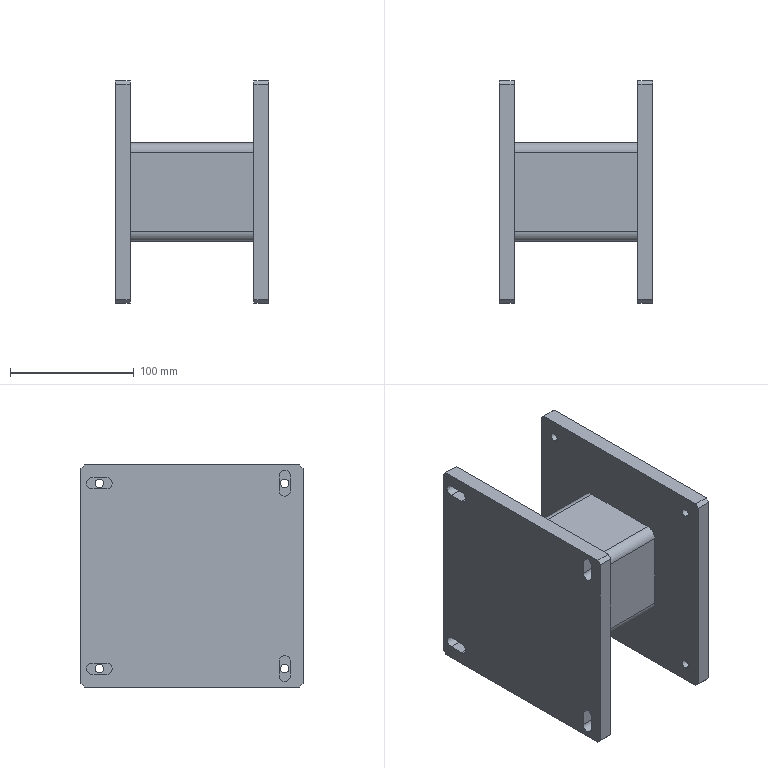Part | STEP file | PN_0063_Default<machined> | 3 solids | 64 faces | box 124 x 180 x 180 mm | volume 884667 mm3 | plane 38 | cylinder 26 | commonest cylinder face diameters 9 x10 6.8 x8 8 x4 16 x4